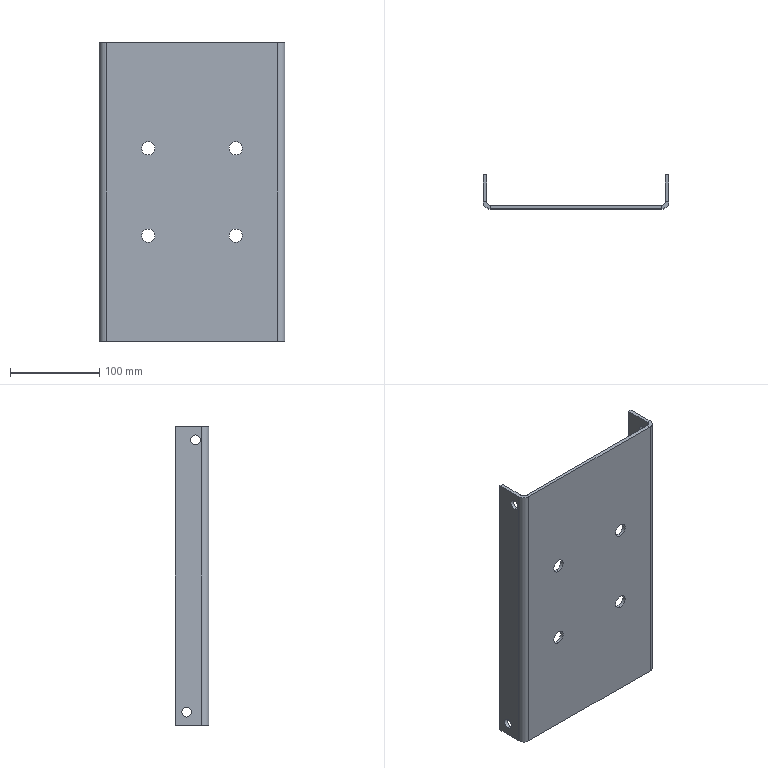Part | SolidWorks | features Cut 1, FlatPattern 1, ICE 1, SMBaseFlange 1, SheetMetal 1 | 1 solid | 38 faces | box 208 x 38 x 335 mm | volume 358590 mm3 | cylinder 20 | plane 18 | commonest cylinder face diameters 11 x8 15 x8 8 x2 16 x2
STEP:
#1=CARTESIAN_POINT('',(-49.,0.,-56.5));
#2=VERTEX_POINT('',#1);
#3=CARTESIAN_POINT('',(-49.,0.,-41.5));
#4=VERTEX_POINT('',#3);
#5=CARTESIAN_POINT('',(-49.,0.,-49.));
#6=DIRECTION('',(0.,1.,0.));
#7=DIRECTION('',(0.,0.,1.));
#8=AXIS2_PLACEMENT_3D('',#5,#6,#7);
#9=CIRCLE('',#8,7.5);
#10=EDGE_CURVE('',#2,#4,#9,.T.);
#11=ORIENTED_EDGE('',*,*,#10,.F.);
#12=CARTESIAN_POINT('',(-49.,4.,-56.5));
#13=VERTEX_POINT('',#12);
#14=CARTESIAN_POINT('',(-49.,-6.,-56.5));
#15=DIRECTION('',(0.,1.,0.));
#16=VECTOR('',#15,1000.);
#17=LINE('',#14,#16);
#18=EDGE_CURVE('',#2,#13,#17,.T.);
#19=ORIENTED_EDGE('',*,*,#18,.T.);
#20=CARTESIAN_POINT('',(-49.,4.,-41.5));
#21=VERTEX_POINT('',#20);
#22=CARTESIAN_POINT('',(-49.,4.,-49.));
#23=DIRECTION('',(0.,1.,0.));
#24=DIRECTION('',(0.,0.,1.));
#25=AXIS2_PLACEMENT_3D('',#22,#23,#24);
#26=CIRCLE('',#25,7.5);
#27=EDGE_CURVE('',#13,#21,#26,.T.);
#28=ORIENTED_EDGE('',*,*,#27,.T.);
#29=CARTESIAN_POINT('',(-49.,-6.,-41.5));
#30=DIRECTION('',(0.,1.,0.));
#31=VECTOR('',#30,1000.);
#32=LINE('',#29,#31);
#33=EDGE_CURVE('',#4,#21,#32,.T.);
#34=ORIENTED_EDGE('',*,*,#33,.F.);
#35=EDGE_LOOP('',(#11,#19,#28,#34));
#36=FACE_OUTER_BOUND('',#35,.T.);
#37=CARTESIAN_POINT('',(-49.,-6.,-49.));
#38=DIRECTION('',(0.,1.,0.));
#39=DIRECTION('',(0.,0.,1.));
#40=AXIS2_PLACEMENT_3D('',#37,#38,#39);
#41=CYLINDRICAL_SURFACE('',#40,7.5);
#42=ADVANCED_FACE('',(#36),#41,.F.);
#43=CARTESIAN_POINT('',(49.,0.,41.5));
#44=VERTEX_POINT('',#43);
#45=CARTESIAN_POINT('',(49.,0.,56.5));
#46=VERTEX_POINT('',#45);
#47=CARTESIAN_POINT('',(49.,0.,49.));
#48=DIRECTION('',(0.,1.,0.));
#49=DIRECTION('',(0.,0.,1.));
#50=AXIS2_PLACEMENT_3D('',#47,#48,#49);
#51=CIRCLE('',#50,7.5);
#52=EDGE_CURVE('',#44,#46,#51,.T.);
#53=ORIENTED_EDGE('',*,*,#52,.F.);
#54=CARTESIAN_POINT('',(49.,4.,41.5));
#55=VERTEX_POINT('',#54);
#56=CARTESIAN_POINT('',(49.,-6.,41.5));
#57=DIRECTION('',(0.,1.,0.));
#58=VECTOR('',#57,1000.);
#59=LINE('',#56,#58);
#60=EDGE_CURVE('',#44,#55,#59,.T.);
#61=ORIENTED_EDGE('',*,*,#60,.T.);
#62=CARTESIAN_POINT('',(49.,4.,56.5));
#63=VERTEX_POINT('',#62);
#64=CARTESIAN_POINT('',(49.,4.,49.));
#65=DIRECTION('',(0.,1.,0.));
#66=DIRECTION('',(0.,0.,1.));
#67=AXIS2_PLACEMENT_3D('',#64,#65,#66);
#68=CIRCLE('',#67,7.5);
#69=EDGE_CURVE('',#55,#63,#68,.T.);
#70=ORIENTED_EDGE('',*,*,#69,.T.);
#71=CARTESIAN_POINT('',(49.,-6.,56.5));
#72=DIRECTION('',(0.,1.,0.));
#73=VECTOR('',#72,1000.);
#74=LINE('',#71,#73);
#75=EDGE_CURVE('',#46,#63,#74,.T.);
#76=ORIENTED_EDGE('',*,*,#75,.F.);
#77=EDGE_LOOP('',(#53,#61,#70,#76));
#78=FACE_OUTER_BOUND('',#77,.T.);
#79=CARTESIAN_POINT('',(49.,-6.,49.));
#80=DIRECTION('',(0.,1.,0.));
#81=DIRECTION('',(0.,0.,1.));
#82=AXIS2_PLACEMENT_3D('',#79,#80,#81);
#83=CYLINDRICAL_SURFACE('',#82,7.5);
#84=ADVANCED_FACE('',(#78),#83,.F.);
#85=CARTESIAN_POINT('',(-49.,0.,41.5));
#86=VERTEX_POINT('',#85);
#87=CARTESIAN_POINT('',(-49.,0.,56.5));
#88=VERTEX_POINT('',#87);
#89=CARTESIAN_POINT('',(-49.,0.,49.));
#90=DIRECTION('',(0.,1.,0.));
#91=DIRECTION('',(0.,0.,1.));
#92=AXIS2_PLACEMENT_3D('',#89,#90,#91);
#93=CIRCLE('',#92,7.5);
#94=EDGE_CURVE('',#86,#88,#93,.T.);
#95=ORIENTED_EDGE('',*,*,#94,.F.);
#96=CARTESIAN_POINT('',(-49.,4.,41.5));
#97=VERTEX_POINT('',#96);
#98=CARTESIAN_POINT('',(-49.,-6.,41.5));
#99=DIRECTION('',(0.,1.,0.));
#100=VECTOR('',#99,1000.);
#101=LINE('',#98,#100);
#102=EDGE_CURVE('',#86,#97,#101,.T.);
#103=ORIENTED_EDGE('',*,*,#102,.T.);
#104=CARTESIAN_POINT('',(-49.,4.,56.5));
#105=VERTEX_POINT('',#104);
#106=CARTESIAN_POINT('',(-49.,4.,49.));
#107=DIRECTION('',(0.,1.,0.));
#108=DIRECTION('',(0.,0.,1.));
#109=AXIS2_PLACEMENT_3D('',#106,#107,#108);
#110=CIRCLE('',#109,7.5);
#111=EDGE_CURVE('',#97,#105,#110,.T.);
#112=ORIENTED_EDGE('',*,*,#111,.T.);
#113=CARTESIAN_POINT('',(-49.,-6.,56.5));
#114=DIRECTION('',(0.,1.,0.));
#115=VECTOR('',#114,1000.);
#116=LINE('',#113,#115);
#117=EDGE_CURVE('',#88,#105,#116,.T.);
#118=ORIENTED_EDGE('',*,*,#117,.F.);
#119=EDGE_LOOP('',(#95,#103,#112,#118));
#120=FACE_OUTER_BOUND('',#119,.T.);
#121=CARTESIAN_POINT('',(-49.,-6.,49.));
#122=DIRECTION('',(0.,1.,0.));
#123=DIRECTION('',(0.,0.,1.));
#124=AXIS2_PLACEMENT_3D('',#121,#122,#123);
#125=CYLINDRICAL_SURFACE('',#124,7.5);
#126=ADVANCED_FACE('',(#120),#125,.F.);
#127=CARTESIAN_POINT('',(49.,0.,-56.5));
#128=VERTEX_POINT('',#127);
#129=CARTESIAN_POINT('',(49.,0.,-41.5));
#130=VERTEX_POINT('',#129);
#131=CARTESIAN_POINT('',(49.,0.,-49.));
#132=DIRECTION('',(0.,1.,0.));
#133=DIRECTION('',(0.,0.,1.));
#134=AXIS2_PLACEMENT_3D('',#131,#132,#133);
#135=CIRCLE('',#134,7.5);
#136=EDGE_CURVE('',#128,#130,#135,.T.);
#137=ORIENTED_EDGE('',*,*,#136,.F.);
#138=CARTESIAN_POINT('',(49.,4.,-56.5));
#139=VERTEX_POINT('',#138);
#140=CARTESIAN_POINT('',(49.,-6.,-56.5));
#141=DIRECTION('',(0.,1.,0.));
#142=VECTOR('',#141,1000.);
#143=LINE('',#140,#142);
#144=EDGE_CURVE('',#128,#139,#143,.T.);
#145=ORIENTED_EDGE('',*,*,#144,.T.);
#146=CARTESIAN_POINT('',(49.,4.,-41.5));
#147=VERTEX_POINT('',#146);
#148=CARTESIAN_POINT('',(49.,4.,-49.));
#149=DIRECTION('',(0.,1.,0.));
#150=DIRECTION('',(0.,0.,1.));
#151=AXIS2_PLACEMENT_3D('',#148,#149,#150);
#152=CIRCLE('',#151,7.5);
#153=EDGE_CURVE('',#139,#147,#152,.T.);
#154=ORIENTED_EDGE('',*,*,#153,.T.);
#155=CARTESIAN_POINT('',(49.,-6.,-41.5));
#156=DIRECTION('',(0.,1.,0.));
#157=VECTOR('',#156,1000.);
#158=LINE('',#155,#157);
#159=EDGE_CURVE('',#130,#147,#158,.T.);
#160=ORIENTED_EDGE('',*,*,#159,.F.);
#161=EDGE_LOOP('',(#137,#145,#154,#160));
#162=FACE_OUTER_BOUND('',#161,.T.);
#163=CARTESIAN_POINT('',(49.,-6.,-49.));
#164=DIRECTION('',(0.,1.,0.));
#165=DIRECTION('',(0.,0.,1.));
#166=AXIS2_PLACEMENT_3D('',#163,#164,#165);
#167=CYLINDRICAL_SURFACE('',#166,7.5);
#168=ADVANCED_FACE('',(#162),#167,.F.);
#169=CARTESIAN_POINT('',(104.,25.,-158.));
#170=VERTEX_POINT('',#169);
#171=CARTESIAN_POINT('',(104.,25.,-147.));
#172=VERTEX_POINT('',#171);
#173=CARTESIAN_POINT('',(104.,25.,-152.5));
#174=DIRECTION('',(-1.,0.,0.));
#175=DIRECTION('',(0.,0.,1.));
#176=AXIS2_PLACEMENT_3D('',#173,#174,#175);
#177=CIRCLE('',#176,5.5);
#178=EDGE_CURVE('',#170,#172,#177,.T.);
#179=ORIENTED_EDGE('',*,*,#178,.F.);
#180=CARTESIAN_POINT('',(100.,25.,-158.));
#181=VERTEX_POINT('',#180);
#182=CARTESIAN_POINT('',(104.,25.,-158.));
#183=DIRECTION('',(-1.,0.,0.));
#184=VECTOR('',#183,1000.);
#185=LINE('',#182,#184);
#186=EDGE_CURVE('',#170,#181,#185,.T.);
#187=ORIENTED_EDGE('',*,*,#186,.T.);
#188=CARTESIAN_POINT('',(100.,25.,-147.));
#189=VERTEX_POINT('',#188);
#190=CARTESIAN_POINT('',(100.,25.,-152.5));
#191=DIRECTION('',(-1.,0.,0.));
#192=DIRECTION('',(0.,0.,1.));
#193=AXIS2_PLACEMENT_3D('',#190,#191,#192);
#194=CIRCLE('',#193,5.5);
#195=EDGE_CURVE('',#181,#189,#194,.T.);
#196=ORIENTED_EDGE('',*,*,#195,.T.);
#197=CARTESIAN_POINT('',(104.,25.,-147.));
#198=DIRECTION('',(-1.,0.,0.));
#199=VECTOR('',#198,1000.);
#200=LINE('',#197,#199);
#201=EDGE_CURVE('',#172,#189,#200,.T.);
#202=ORIENTED_EDGE('',*,*,#201,.F.);
#203=EDGE_LOOP('',(#179,#187,#196,#202));
#204=FACE_OUTER_BOUND('',#203,.T.);
#205=CARTESIAN_POINT('',(104.,25.,-152.5));
#206=DIRECTION('',(-1.,0.,0.));
#207=DIRECTION('',(0.,0.,1.));
#208=AXIS2_PLACEMENT_3D('',#205,#206,#207);
#209=CYLINDRICAL_SURFACE('',#208,5.5);
#210=ADVANCED_FACE('',(#204),#209,.F.);
#211=CARTESIAN_POINT('',(104.,15.,147.));
#212=VERTEX_POINT('',#211);
#213=CARTESIAN_POINT('',(104.,15.,158.));
#214=VERTEX_POINT('',#213);
#215=CARTESIAN_POINT('',(104.,15.,152.5));
#216=DIRECTION('',(-1.,0.,0.));
#217=DIRECTION('',(0.,0.,1.));
#218=AXIS2_PLACEMENT_3D('',#215,#216,#217);
#219=CIRCLE('',#218,5.5);
#220=EDGE_CURVE('',#212,#214,#219,.T.);
#221=ORIENTED_EDGE('',*,*,#220,.F.);
#222=CARTESIAN_POINT('',(100.,15.,147.));
#223=VERTEX_POINT('',#222);
#224=CARTESIAN_POINT('',(104.,15.,147.));
#225=DIRECTION('',(-1.,0.,0.));
#226=VECTOR('',#225,1000.);
#227=LINE('',#224,#226);
#228=EDGE_CURVE('',#212,#223,#227,.T.);
#229=ORIENTED_EDGE('',*,*,#228,.T.);
#230=CARTESIAN_POINT('',(100.,15.,158.));
#231=VERTEX_POINT('',#230);
#232=CARTESIAN_POINT('',(100.,15.,152.5));
#233=DIRECTION('',(-1.,0.,0.));
#234=DIRECTION('',(0.,0.,1.));
#235=AXIS2_PLACEMENT_3D('',#232,#233,#234);
#236=CIRCLE('',#235,5.5);
#237=EDGE_CURVE('',#223,#231,#236,.T.);
#238=ORIENTED_EDGE('',*,*,#237,.T.);
#239=CARTESIAN_POINT('',(104.,15.,158.));
#240=DIRECTION('',(-1.,0.,0.));
#241=VECTOR('',#240,1000.);
#242=LINE('',#239,#241);
#243=EDGE_CURVE('',#214,#231,#242,.T.);
#244=ORIENTED_EDGE('',*,*,#243,.F.);
#245=EDGE_LOOP('',(#221,#229,#238,#244));
#246=FACE_OUTER_BOUND('',#245,.T.);
#247=CARTESIAN_POINT('',(104.,15.,152.5));
#248=DIRECTION('',(-1.,0.,0.));
#249=DIRECTION('',(0.,0.,1.));
#250=AXIS2_PLACEMENT_3D('',#247,#248,#249);
#251=CYLINDRICAL_SURFACE('',#250,5.5);
#252=ADVANCED_FACE('',(#246),#251,.F.);
#253=CARTESIAN_POINT('',(-100.,25.,-147.));
#254=VERTEX_POINT('',#253);
#255=CARTESIAN_POINT('',(-100.,25.,-158.));
#256=VERTEX_POINT('',#255);
#257=CARTESIAN_POINT('',(-100.,25.,-152.5));
#258=DIRECTION('',(1.,0.,0.));
#259=DIRECTION('',(0.,0.,-1.));
#260=AXIS2_PLACEMENT_3D('',#257,#258,#259);
#261=CIRCLE('',#260,5.5);
#262=EDGE_CURVE('',#254,#256,#261,.T.);
#263=ORIENTED_EDGE('',*,*,#262,.T.);
#264=CARTESIAN_POINT('',(-104.,25.,-158.));
#265=VERTEX_POINT('',#264);
#266=CARTESIAN_POINT('',(104.,25.,-158.));
#267=DIRECTION('',(-1.,0.,0.));
#268=VECTOR('',#267,1000.);
#269=LINE('',#266,#268);
#270=EDGE_CURVE('',#256,#265,#269,.T.);
#271=ORIENTED_EDGE('',*,*,#270,.T.);
#272=CARTESIAN_POINT('',(-104.,25.,-147.));
#273=VERTEX_POINT('',#272);
#274=CARTESIAN_POINT('',(-104.,25.,-152.5));
#275=DIRECTION('',(1.,0.,0.));
#276=DIRECTION('',(0.,0.,-1.));
#277=AXIS2_PLACEMENT_3D('',#274,#275,#276);
#278=CIRCLE('',#277,5.5);
#279=EDGE_CURVE('',#273,#265,#278,.T.);
#280=ORIENTED_EDGE('',*,*,#279,.F.);
#281=CARTESIAN_POINT('',(104.,25.,-147.));
#282=DIRECTION('',(-1.,0.,0.));
#283=VECTOR('',#282,1000.);
#284=LINE('',#281,#283);
#285=EDGE_CURVE('',#254,#273,#284,.T.);
#286=ORIENTED_EDGE('',*,*,#285,.F.);
#287=EDGE_LOOP('',(#263,#271,#280,#286));
#288=FACE_OUTER_BOUND('',#287,.T.);
#289=CARTESIAN_POINT('',(104.,25.,-152.5));
#290=DIRECTION('',(-1.,0.,0.));
#291=DIRECTION('',(0.,0.,1.));
#292=AXIS2_PLACEMENT_3D('',#289,#290,#291);
#293=CYLINDRICAL_SURFACE('',#292,5.5);
#294=ADVANCED_FACE('',(#288),#293,.F.);
#295=CARTESIAN_POINT('',(-100.,15.,158.));
#296=VERTEX_POINT('',#295);
#297=CARTESIAN_POINT('',(-100.,15.,147.));
#298=VERTEX_POINT('',#297);
#299=CARTESIAN_POINT('',(-100.,15.,152.5));
#300=DIRECTION('',(1.,0.,0.));
#301=DIRECTION('',(0.,0.,-1.));
#302=AXIS2_PLACEMENT_3D('',#299,#300,#301);
#303=CIRCLE('',#302,5.5);
#304=EDGE_CURVE('',#296,#298,#303,.T.);
#305=ORIENTED_EDGE('',*,*,#304,.T.);
#306=CARTESIAN_POINT('',(-104.,15.,147.));
#307=VERTEX_POINT('',#306);
#308=CARTESIAN_POINT('',(104.,15.,147.));
#309=DIRECTION('',(-1.,0.,0.));
#310=VECTOR('',#309,1000.);
#311=LINE('',#308,#310);
#312=EDGE_CURVE('',#298,#307,#311,.T.);
#313=ORIENTED_EDGE('',*,*,#312,.T.);
#314=CARTESIAN_POINT('',(-104.,15.,158.));
#315=VERTEX_POINT('',#314);
#316=CARTESIAN_POINT('',(-104.,15.,152.5));
#317=DIRECTION('',(1.,0.,0.));
#318=DIRECTION('',(0.,0.,-1.));
#319=AXIS2_PLACEMENT_3D('',#316,#317,#318);
#320=CIRCLE('',#319,5.5);
#321=EDGE_CURVE('',#315,#307,#320,.T.);
#322=ORIENTED_EDGE('',*,*,#321,.F.);
#323=CARTESIAN_POINT('',(104.,15.,158.));
#324=DIRECTION('',(-1.,0.,0.));
#325=VECTOR('',#324,1000.);
#326=LINE('',#323,#325);
#327=EDGE_CURVE('',#296,#315,#326,.T.);
#328=ORIENTED_EDGE('',*,*,#327,.F.);
#329=EDGE_LOOP('',(#305,#313,#322,#328));
#330=FACE_OUTER_BOUND('',#329,.T.);
#331=CARTESIAN_POINT('',(104.,15.,152.5));
#332=DIRECTION('',(-1.,0.,0.));
#333=DIRECTION('',(0.,0.,1.));
#334=AXIS2_PLACEMENT_3D('',#331,#332,#333);
#335=CYLINDRICAL_SURFACE('',#334,5.5);
#336=ADVANCED_FACE('',(#330),#335,.F.);
#337=CARTESIAN_POINT('',(-104.,8.,167.5));
#338=VERTEX_POINT('',#337);
#339=CARTESIAN_POINT('',(-100.,8.,167.5));
#340=VERTEX_POINT('',#339);
#341=CARTESIAN_POINT('',(-104.,8.,167.5));
#342=DIRECTION('',(1.,0.,0.));
#343=VECTOR('',#342,1000.);
#344=LINE('',#341,#343);
#345=EDGE_CURVE('',#338,#340,#344,.T.);
#346=ORIENTED_EDGE('',*,*,#345,.F.);
#347=CARTESIAN_POINT('',(-96.,0.,167.5));
#348=VERTEX_POINT('',#347);
#349=CARTESIAN_POINT('',(-96.,8.,167.5));
#350=DIRECTION('',(0.,0.,1.));
#351=DIRECTION('',(-1.,0.,0.));
#352=AXIS2_PLACEMENT_3D('',#349,#350,#351);
#353=CIRCLE('',#352,8.);
#354=EDGE_CURVE('',#338,#348,#353,.T.);
#355=ORIENTED_EDGE('',*,*,#354,.T.);
#356=CARTESIAN_POINT('',(-96.,4.,167.5));
#357=VERTEX_POINT('',#356);
#358=CARTESIAN_POINT('',(-96.,4.,167.5));
#359=DIRECTION('',(0.,-1.,0.));
#360=VECTOR('',#359,1000.);
#361=LINE('',#358,#360);
#362=EDGE_CURVE('',#357,#348,#361,.T.);
#363=ORIENTED_EDGE('',*,*,#362,.F.);
#364=CARTESIAN_POINT('',(-96.,8.,167.5));
#365=DIRECTION('',(0.,0.,1.));
#366=DIRECTION('',(1.,0.,0.));
#367=AXIS2_PLACEMENT_3D('',#364,#365,#366);
#368=CIRCLE('',#367,4.);
#369=EDGE_CURVE('',#340,#357,#368,.T.);
#370=ORIENTED_EDGE('',*,*,#369,.F.);
#371=EDGE_LOOP('',(#346,#355,#363,#370));
#372=FACE_OUTER_BOUND('',#371,.T.);
#373=CARTESIAN_POINT('',(-104.,8.,167.5));
#374=DIRECTION('',(0.,0.,1.));
#375=DIRECTION('',(1.,0.,0.));
#376=AXIS2_PLACEMENT_3D('',#373,#374,#375);
#377=PLANE('',#376);
#378=ADVANCED_FACE('',(#372),#377,.T.);
#379=CARTESIAN_POINT('',(-104.,38.,167.5));
#380=VERTEX_POINT('',#379);
#381=CARTESIAN_POINT('',(-104.,38.,167.5));
#382=DIRECTION('',(0.,-1.,0.));
#383=VECTOR('',#382,1000.);
#384=LINE('',#381,#383);
#385=EDGE_CURVE('',#380,#338,#384,.T.);
#386=ORIENTED_EDGE('',*,*,#385,.T.);
#387=ORIENTED_EDGE('',*,*,#345,.T.);
#388=CARTESIAN_POINT('',(-100.,38.,167.5));
#389=VERTEX_POINT('',#388);
#390=CARTESIAN_POINT('',(-100.,38.,167.5));
#391=DIRECTION('',(0.,-1.,0.));
#392=VECTOR('',#391,1000.);
#393=LINE('',#390,#392);
#394=EDGE_CURVE('',#389,#340,#393,.T.);
#395=ORIENTED_EDGE('',*,*,#394,.F.);
#396=CARTESIAN_POINT('',(-104.,38.,167.5));
#397=DIRECTION('',(1.,0.,0.));
#398=VECTOR('',#397,1000.);
#399=LINE('',#396,#398);
#400=EDGE_CURVE('',#380,#389,#399,.T.);
#401=ORIENTED_EDGE('',*,*,#400,.F.);
#402=EDGE_LOOP('',(#386,#387,#395,#401));
#403=FACE_OUTER_BOUND('',#402,.T.);
#404=CARTESIAN_POINT('',(-96.,4.,167.5));
#405=DIRECTION('',(0.,0.,1.));
#406=DIRECTION('',(1.,0.,0.));
#407=AXIS2_PLACEMENT_3D('',#404,#405,#406);
#408=PLANE('',#407);
#409=ADVANCED_FACE('',(#403),#408,.T.);
#410=CARTESIAN_POINT('',(-96.,0.,-167.5));
#411=VERTEX_POINT('',#410);
#412=CARTESIAN_POINT('',(-96.,4.,-167.5));
#413=VERTEX_POINT('',#412);
#414=CARTESIAN_POINT('',(-96.,0.,-167.5));
#415=DIRECTION('',(0.,1.,0.));
#416=VECTOR('',#415,1000.);
#417=LINE('',#414,#416);
#418=EDGE_CURVE('',#411,#413,#417,.T.);
#419=ORIENTED_EDGE('',*,*,#418,.F.);
#420=CARTESIAN_POINT('',(-104.,8.,-167.5));
#421=VERTEX_POINT('',#420);
#422=CARTESIAN_POINT('',(-96.,8.,-167.5));
#423=DIRECTION('',(0.,0.,1.));
#424=DIRECTION('',(-1.,0.,0.));
#425=AXIS2_PLACEMENT_3D('',#422,#423,#424);
#426=CIRCLE('',#425,8.);
#427=EDGE_CURVE('',#421,#411,#426,.T.);
#428=ORIENTED_EDGE('',*,*,#427,.F.);
#429=CARTESIAN_POINT('',(-100.,8.,-167.5));
#430=VERTEX_POINT('',#429);
#431=CARTESIAN_POINT('',(-100.,8.,-167.5));
#432=DIRECTION('',(-1.,0.,0.));
#433=VECTOR('',#432,1000.);
#434=LINE('',#431,#433);
#435=EDGE_CURVE('',#430,#421,#434,.T.);
#436=ORIENTED_EDGE('',*,*,#435,.F.);
#437=CARTESIAN_POINT('',(-96.,8.,-167.5));
#438=DIRECTION('',(0.,0.,1.));
#439=DIRECTION('',(1.,0.,0.));
#440=AXIS2_PLACEMENT_3D('',#437,#438,#439);
#441=CIRCLE('',#440,4.);
#442=EDGE_CURVE('',#430,#413,#441,.T.);
#443=ORIENTED_EDGE('',*,*,#442,.T.);
#444=EDGE_LOOP('',(#419,#428,#436,#443));
#445=FACE_OUTER_BOUND('',#444,.T.);
#446=CARTESIAN_POINT('',(-96.,0.,-167.5));
#447=DIRECTION('',(0.,0.,-1.));
#448=DIRECTION('',(-1.,0.,0.));
#449=AXIS2_PLACEMENT_3D('',#446,#447,#448);
#450=PLANE('',#449);
#451=ADVANCED_FACE('',(#445),#450,.T.);
#452=CARTESIAN_POINT('',(96.,0.,-167.5));
#453=VERTEX_POINT('',#452);
#454=CARTESIAN_POINT('',(-104.,0.,-167.5));
#455=DIRECTION('',(1.,0.,0.));
#456=VECTOR('',#455,1000.);
#457=LINE('',#454,#456);
#458=EDGE_CURVE('',#411,#453,#457,.T.);
#459=ORIENTED_EDGE('',*,*,#458,.F.);
#460=ORIENTED_EDGE('',*,*,#418,.T.);
#461=CARTESIAN_POINT('',(96.,4.,-167.5));
#462=VERTEX_POINT('',#461);
#463=CARTESIAN_POINT('',(-104.,4.,-167.5));
#464=DIRECTION('',(1.,0.,0.));
#465=VECTOR('',#464,1000.);
#466=LINE('',#463,#465);
#467=EDGE_CURVE('',#413,#462,#466,.T.);
#468=ORIENTED_EDGE('',*,*,#467,.T.);
#469=CARTESIAN_POINT('',(96.,4.,-167.5));
#470=DIRECTION('',(0.,-1.,0.));
#471=VECTOR('',#470,1000.);
#472=LINE('',#469,#471);
#473=EDGE_CURVE('',#462,#453,#472,.T.);
#474=ORIENTED_EDGE('',*,*,#473,.T.);
#475=EDGE_LOOP('',(#459,#460,#468,#474));
#476=FACE_OUTER_BOUND('',#475,.T.);
#477=CARTESIAN_POINT('',(-100.,8.,-167.5));
#478=DIRECTION('',(0.,0.,-1.));
#479=DIRECTION('',(-1.,0.,0.));
#480=AXIS2_PLACEMENT_3D('',#477,#478,#479);
#481=PLANE('',#480);
#482=ADVANCED_FACE('',(#476),#481,.T.);
#483=CARTESIAN_POINT('',(96.,0.,167.5));
#484=VERTEX_POINT('',#483);
#485=CARTESIAN_POINT('',(96.,4.,167.5));
#486=VERTEX_POINT('',#485);
#487=CARTESIAN_POINT('',(96.,0.,167.5));
#488=DIRECTION('',(0.,1.,0.));
#489=VECTOR('',#488,1000.);
#490=LINE('',#487,#489);
#491=EDGE_CURVE('',#484,#486,#490,.T.);
#492=ORIENTED_EDGE('',*,*,#491,.F.);
#493=CARTESIAN_POINT('',(104.,8.,167.5));
#494=VERTEX_POINT('',#493);
#495=CARTESIAN_POINT('',(96.,8.,167.5));
#496=DIRECTION('',(0.,0.,1.));
#497=DIRECTION('',(-1.,0.,0.));
#498=AXIS2_PLACEMENT_3D('',#495,#496,#497);
#499=CIRCLE('',#498,8.);
#500=EDGE_CURVE('',#484,#494,#499,.T.);
#501=ORIENTED_EDGE('',*,*,#500,.T.);
#502=CARTESIAN_POINT('',(100.,8.,167.5));
#503=VERTEX_POINT('',#502);
#504=CARTESIAN_POINT('',(100.,8.,167.5));
#505=DIRECTION('',(1.,0.,0.));
#506=VECTOR('',#505,1000.);
#507=LINE('',#504,#506);
#508=EDGE_CURVE('',#503,#494,#507,.T.);
#509=ORIENTED_EDGE('',*,*,#508,.F.);
#510=CARTESIAN_POINT('',(96.,8.,167.5));
#511=DIRECTION('',(0.,0.,1.));
#512=DIRECTION('',(1.,0.,0.));
#513=AXIS2_PLACEMENT_3D('',#510,#511,#512);
#514=CIRCLE('',#513,4.);
#515=EDGE_CURVE('',#486,#503,#514,.T.);
#516=ORIENTED_EDGE('',*,*,#515,.F.);
#517=EDGE_LOOP('',(#492,#501,#509,#516));
#518=FACE_OUTER_BOUND('',#517,.T.);
#519=CARTESIAN_POINT('',(96.,0.,167.5));
#520=DIRECTION('',(0.,0.,1.));
#521=DIRECTION('',(1.,0.,0.));
#522=AXIS2_PLACEMENT_3D('',#519,#520,#521);
#523=PLANE('',#522);
#524=ADVANCED_FACE('',(#518),#523,.T.);
#525=CARTESIAN_POINT('',(-104.,0.,167.5));
#526=DIRECTION('',(1.,0.,0.));
#527=VECTOR('',#526,1000.);
#528=LINE('',#525,#527);
#529=EDGE_CURVE('',#348,#484,#528,.T.);
#530=ORIENTED_EDGE('',*,*,#529,.T.);
#531=ORIENTED_EDGE('',*,*,#491,.T.);
#532=CARTESIAN_POINT('',(-104.,4.,167.5));
#533=DIRECTION('',(1.,0.,0.));
#534=VECTOR('',#533,1000.);
#535=LINE('',#532,#534);
#536=EDGE_CURVE('',#357,#486,#535,.T.);
#537=ORIENTED_EDGE('',*,*,#536,.F.);
#538=ORIENTED_EDGE('',*,*,#362,.T.);
#539=EDGE_LOOP('',(#530,#531,#537,#538));
#540=FACE_OUTER_BOUND('',#539,.T.);
#541=CARTESIAN_POINT('',(100.,8.,167.5));
#542=DIRECTION('',(0.,0.,1.));
#543=DIRECTION('',(1.,0.,0.));
#544=AXIS2_PLACEMENT_3D('',#541,#542,#543);
#545=PLANE('',#544);
#546=ADVANCED_FACE('',(#540),#545,.T.);
#547=CARTESIAN_POINT('',(104.,8.,-167.5));
#548=VERTEX_POINT('',#547);
#549=CARTESIAN_POINT('',(100.,8.,-167.5));
#550=VERTEX_POINT('',#549);
#551=CARTESIAN_POINT('',(104.,8.,-167.5));
#552=DIRECTION('',(-1.,0.,0.));
#553=VECTOR('',#552,1000.);
#554=LINE('',#551,#553);
#555=EDGE_CURVE('',#548,#550,#554,.T.);
#556=ORIENTED_EDGE('',*,*,#555,.F.);
#557=CARTESIAN_POINT('',(96.,8.,-167.5));
#558=DIRECTION('',(0.,0.,1.));
#559=DIRECTION('',(-1.,0.,0.));
#560=AXIS2_PLACEMENT_3D('',#557,#558,#559);
#561=CIRCLE('',#560,8.);
#562=EDGE_CURVE('',#453,#548,#561,.T.);
#563=ORIENTED_EDGE('',*,*,#562,.F.);
#564=ORIENTED_EDGE('',*,*,#473,.F.);
#565=CARTESIAN_POINT('',(96.,8.,-167.5));
#566=DIRECTION('',(0.,0.,1.));
#567=DIRECTION('',(1.,0.,0.));
#568=AXIS2_PLACEMENT_3D('',#565,#566,#567);
#569=CIRCLE('',#568,4.);
#570=EDGE_CURVE('',#462,#550,#569,.T.);
#571=ORIENTED_EDGE('',*,*,#570,.T.);
#572=EDGE_LOOP('',(#556,#563,#564,#571));
#573=FACE_OUTER_BOUND('',#572,.T.);
#574=CARTESIAN_POINT('',(104.,8.,-167.5));
#575=DIRECTION('',(0.,0.,-1.));
#576=DIRECTION('',(-1.,0.,0.));
#577=AXIS2_PLACEMENT_3D('',#574,#575,#576);
#578=PLANE('',#577);
#579=ADVANCED_FACE('',(#573),#578,.T.);
#580=CARTESIAN_POINT('',(104.,38.,-167.5));
#581=VERTEX_POINT('',#580);
#582=CARTESIAN_POINT('',(104.,0.,-167.5));
#583=DIRECTION('',(0.,1.,0.));
#584=VECTOR('',#583,1000.);
#585=LINE('',#582,#584);
#586=EDGE_CURVE('',#548,#581,#585,.T.);
#587=ORIENTED_EDGE('',*,*,#586,.F.);
#588=ORIENTED_EDGE('',*,*,#555,.T.);
#589=CARTESIAN_POINT('',(100.,38.,-167.5));
#590=VERTEX_POINT('',#589);
#591=CARTESIAN_POINT('',(100.,0.,-167.5));
#592=DIRECTION('',(0.,1.,0.));
#593=VECTOR('',#592,1000.);
#594=LINE('',#591,#593);
#595=EDGE_CURVE('',#550,#590,#594,.T.);
#596=ORIENTED_EDGE('',*,*,#595,.T.);
#597=CARTESIAN_POINT('',(100.,38.,-167.5));
#598=DIRECTION('',(1.,0.,0.));
#599=VECTOR('',#598,1000.);
#600=LINE('',#597,#599);
#601=EDGE_CURVE('',#590,#581,#600,.T.);
#602=ORIENTED_EDGE('',*,*,#601,.T.);
#603=EDGE_LOOP('',(#587,#588,#596,#602));
#604=FACE_OUTER_BOUND('',#603,.T.);
#605=CARTESIAN_POINT('',(96.,4.,-167.5));
#606=DIRECTION('',(0.,0.,-1.));
#607=DIRECTION('',(-1.,0.,0.));
#608=AXIS2_PLACEMENT_3D('',#605,#606,#607);
#609=PLANE('',#608);
#610=ADVANCED_FACE('',(#604),#609,.T.);
#611=CARTESIAN_POINT('',(104.,25.,-152.5));
#612=DIRECTION('',(-1.,0.,0.));
#613=DIRECTION('',(0.,0.,1.));
#614=AXIS2_PLACEMENT_3D('',#611,#612,#613);
#615=CIRCLE('',#614,5.5);
#616=EDGE_CURVE('',#172,#170,#615,.T.);
#617=ORIENTED_EDGE('',*,*,#616,.T.);
#618=ORIENTED_EDGE('',*,*,#178,.T.);
#619=EDGE_LOOP('',(#617,#618));
#620=FACE_BOUND('',#619,.T.);
#621=CARTESIAN_POINT('',(104.,15.,152.5));
#622=DIRECTION('',(-1.,0.,0.));
#623=DIRECTION('',(0.,0.,1.));
#624=AXIS2_PLACEMENT_3D('',#621,#622,#623);
#625=CIRCLE('',#624,5.5);
#626=EDGE_CURVE('',#214,#212,#625,.T.);
#627=ORIENTED_EDGE('',*,*,#626,.T.);
#628=ORIENTED_EDGE('',*,*,#220,.T.);
#629=EDGE_LOOP('',(#627,#628));
#630=FACE_BOUND('',#629,.T.);
#631=ORIENTED_EDGE('',*,*,#586,.T.);
#632=CARTESIAN_POINT('',(104.,38.,167.5));
#633=VERTEX_POINT('',#632);
#634=CARTESIAN_POINT('',(104.,38.,167.5));
#635=DIRECTION('',(0.,0.,-1.));
#636=VECTOR('',#635,1000.);
#637=LINE('',#634,#636);
#638=EDGE_CURVE('',#633,#581,#637,.T.);
#639=ORIENTED_EDGE('',*,*,#638,.F.);
#640=CARTESIAN_POINT('',(104.,0.,167.5));
#641=DIRECTION('',(0.,1.,0.));
#642=VECTOR('',#641,1000.);
#643=LINE('',#640,#642);
#644=EDGE_CURVE('',#494,#633,#643,.T.);
#645=ORIENTED_EDGE('',*,*,#644,.F.);
#646=CARTESIAN_POINT('',(104.,8.,167.5));
#647=DIRECTION('',(0.,0.,-1.));
#648=VECTOR('',#647,1000.);
#649=LINE('',#646,#648);
#650=EDGE_CURVE('',#494,#548,#649,.T.);
#651=ORIENTED_EDGE('',*,*,#650,.T.);
#652=EDGE_LOOP('',(#631,#639,#645,#651));
#653=FACE_OUTER_BOUND('',#652,.T.);
#654=CARTESIAN_POINT('',(104.,0.,167.5));
#655=DIRECTION('',(-1.,0.,0.));
#656=DIRECTION('',(0.,0.,1.));
#657=AXIS2_PLACEMENT_3D('',#654,#655,#656);
#658=PLANE('',#657);
#659=ADVANCED_FACE('',(#620,#630,#653),#658,.F.);
#660=ORIENTED_EDGE('',*,*,#601,.F.);
#661=CARTESIAN_POINT('',(100.,38.,167.5));
#662=VERTEX_POINT('',#661);
#663=CARTESIAN_POINT('',(100.,38.,167.5));
#664=DIRECTION('',(0.,0.,-1.));
#665=VECTOR('',#664,1000.);
#666=LINE('',#663,#665);
#667=EDGE_CURVE('',#662,#590,#666,.T.);
#668=ORIENTED_EDGE('',*,*,#667,.F.);
#669=CARTESIAN_POINT('',(100.,38.,167.5));
#670=DIRECTION('',(1.,0.,0.));
#671=VECTOR('',#670,1000.);
#672=LINE('',#669,#671);
#673=EDGE_CURVE('',#662,#633,#672,.T.);
#674=ORIENTED_EDGE('',*,*,#673,.T.);
#675=ORIENTED_EDGE('',*,*,#638,.T.);
#676=EDGE_LOOP('',(#660,#668,#674,#675));
#677=FACE_OUTER_BOUND('',#676,.T.);
#678=CARTESIAN_POINT('',(100.,38.,167.5));
#679=DIRECTION('',(0.,1.,0.));
#680=DIRECTION('',(0.,0.,1.));
#681=AXIS2_PLACEMENT_3D('',#678,#679,#680);
#682=PLANE('',#681);
#683=ADVANCED_FACE('',(#677),#682,.T.);
#684=CARTESIAN_POINT('',(100.,25.,-152.5));
#685=DIRECTION('',(-1.,0.,0.));
#686=DIRECTION('',(0.,0.,1.));
#687=AXIS2_PLACEMENT_3D('',#684,#685,#686);
#688=CIRCLE('',#687,5.5);
#689=EDGE_CURVE('',#189,#181,#688,.T.);
#690=ORIENTED_EDGE('',*,*,#689,.F.);
#691=ORIENTED_EDGE('',*,*,#195,.F.);
#692=EDGE_LOOP('',(#690,#691));
#693=FACE_BOUND('',#692,.T.);
#694=CARTESIAN_POINT('',(100.,15.,152.5));
#695=DIRECTION('',(-1.,0.,0.));
#696=DIRECTION('',(0.,0.,1.));
#697=AXIS2_PLACEMENT_3D('',#694,#695,#696);
#698=CIRCLE('',#697,5.5);
#699=EDGE_CURVE('',#231,#223,#698,.T.);
#700=ORIENTED_EDGE('',*,*,#699,.F.);
#701=ORIENTED_EDGE('',*,*,#237,.F.);
#702=EDGE_LOOP('',(#700,#701));
#703=FACE_BOUND('',#702,.T.);
#704=ORIENTED_EDGE('',*,*,#595,.F.);
#705=CARTESIAN_POINT('',(100.,8.,167.5));
#706=DIRECTION('',(0.,0.,-1.));
#707=VECTOR('',#706,1000.);
#708=LINE('',#705,#707);
#709=EDGE_CURVE('',#503,#550,#708,.T.);
#710=ORIENTED_EDGE('',*,*,#709,.F.);
#711=CARTESIAN_POINT('',(100.,0.,167.5));
#712=DIRECTION('',(0.,1.,0.));
#713=VECTOR('',#712,1000.);
#714=LINE('',#711,#713);
#715=EDGE_CURVE('',#503,#662,#714,.T.);
#716=ORIENTED_EDGE('',*,*,#715,.T.);
#717=ORIENTED_EDGE('',*,*,#667,.T.);
#718=EDGE_LOOP('',(#704,#710,#716,#717));
#719=FACE_OUTER_BOUND('',#718,.T.);
#720=CARTESIAN_POINT('',(100.,0.,167.5));
#721=DIRECTION('',(-1.,0.,0.));
#722=DIRECTION('',(0.,0.,1.));
#723=AXIS2_PLACEMENT_3D('',#720,#721,#722);
#724=PLANE('',#723);
#725=ADVANCED_FACE('',(#693,#703,#719),#724,.T.);
#726=ORIENTED_EDGE('',*,*,#570,.F.);
#727=CARTESIAN_POINT('',(96.,4.,167.5));
#728=DIRECTION('',(0.,0.,-1.));
#729=VECTOR('',#728,1000.);
#730=LINE('',#727,#729);
#731=EDGE_CURVE('',#486,#462,#730,.T.);
#732=ORIENTED_EDGE('',*,*,#731,.F.);
#733=ORIENTED_EDGE('',*,*,#515,.T.);
#734=ORIENTED_EDGE('',*,*,#709,.T.);
#735=EDGE_LOOP('',(#726,#732,#733,#734));
#736=FACE_OUTER_BOUND('',#735,.T.);
#737=CARTESIAN_POINT('',(96.,8.,167.5));
#738=DIRECTION('',(0.,0.,-1.));
#739=DIRECTION('',(-1.,0.,0.));
#740=AXIS2_PLACEMENT_3D('',#737,#738,#739);
#741=CYLINDRICAL_SURFACE('',#740,4.);
#742=ADVANCED_FACE('',(#736),#741,.F.);
#743=CARTESIAN_POINT('',(-49.,4.,-49.));
#744=DIRECTION('',(0.,1.,0.));
#745=DIRECTION('',(0.,0.,1.));
#746=AXIS2_PLACEMENT_3D('',#743,#744,#745);
#747=CIRCLE('',#746,7.5);
#748=EDGE_CURVE('',#21,#13,#747,.T.);
#749=ORIENTED_EDGE('',*,*,#748,.F.);
#750=ORIENTED_EDGE('',*,*,#27,.F.);
#751=EDGE_LOOP('',(#749,#750));
#752=FACE_BOUND('',#751,.T.);
#753=CARTESIAN_POINT('',(49.,4.,49.));
#754=DIRECTION('',(0.,1.,0.));
#755=DIRECTION('',(0.,0.,1.));
#756=AXIS2_PLACEMENT_3D('',#753,#754,#755);
#757=CIRCLE('',#756,7.5);
#758=EDGE_CURVE('',#63,#55,#757,.T.);
#759=ORIENTED_EDGE('',*,*,#758,.F.);
#760=ORIENTED_EDGE('',*,*,#69,.F.);
#761=EDGE_LOOP('',(#759,#760));
#762=FACE_BOUND('',#761,.T.);
#763=CARTESIAN_POINT('',(-49.,4.,49.));
#764=DIRECTION('',(0.,1.,0.));
#765=DIRECTION('',(0.,0.,1.));
#766=AXIS2_PLACEMENT_3D('',#763,#764,#765);
#767=CIRCLE('',#766,7.5);
#768=EDGE_CURVE('',#105,#97,#767,.T.);
#769=ORIENTED_EDGE('',*,*,#768,.F.);
#770=ORIENTED_EDGE('',*,*,#111,.F.);
#771=EDGE_LOOP('',(#769,#770));
#772=FACE_BOUND('',#771,.T.);
#773=CARTESIAN_POINT('',(49.,4.,-49.));
#774=DIRECTION('',(0.,1.,0.));
#775=DIRECTION('',(0.,0.,1.));
#776=AXIS2_PLACEMENT_3D('',#773,#774,#775);
#777=CIRCLE('',#776,7.5);
#778=EDGE_CURVE('',#147,#139,#777,.T.);
#779=ORIENTED_EDGE('',*,*,#778,.F.);
#780=ORIENTED_EDGE('',*,*,#153,.F.);
#781=EDGE_LOOP('',(#779,#780));
#782=FACE_BOUND('',#781,.T.);
#783=ORIENTED_EDGE('',*,*,#467,.F.);
#784=CARTESIAN_POINT('',(-96.,4.,167.5));
#785=DIRECTION('',(0.,0.,-1.));
#786=VECTOR('',#785,1000.);
#787=LINE('',#784,#786);
#788=EDGE_CURVE('',#357,#413,#787,.T.);
#789=ORIENTED_EDGE('',*,*,#788,.F.);
#790=ORIENTED_EDGE('',*,*,#536,.T.);
#791=ORIENTED_EDGE('',*,*,#731,.T.);
#792=EDGE_LOOP('',(#783,#789,#790,#791));
#793=FACE_OUTER_BOUND('',#792,.T.);
#794=CARTESIAN_POINT('',(-104.,4.,167.5));
#795=DIRECTION('',(0.,1.,0.));
#796=DIRECTION('',(0.,0.,1.));
#797=AXIS2_PLACEMENT_3D('',#794,#795,#796);
#798=PLANE('',#797);
#799=ADVANCED_FACE('',(#752,#762,#772,#782,#793),#798,.T.);
#800=ORIENTED_EDGE('',*,*,#442,.F.);
#801=CARTESIAN_POINT('',(-100.,8.,167.5));
#802=DIRECTION('',(0.,0.,-1.));
#803=VECTOR('',#802,1000.);
#804=LINE('',#801,#803);
#805=EDGE_CURVE('',#340,#430,#804,.T.);
#806=ORIENTED_EDGE('',*,*,#805,.F.);
#807=ORIENTED_EDGE('',*,*,#369,.T.);
#808=ORIENTED_EDGE('',*,*,#788,.T.);
#809=EDGE_LOOP('',(#800,#806,#807,#808));
#810=FACE_OUTER_BOUND('',#809,.T.);
#811=CARTESIAN_POINT('',(-96.,8.,167.5));
#812=DIRECTION('',(0.,0.,-1.));
#813=DIRECTION('',(-1.,0.,0.));
#814=AXIS2_PLACEMENT_3D('',#811,#812,#813);
#815=CYLINDRICAL_SURFACE('',#814,4.);
#816=ADVANCED_FACE('',(#810),#815,.F.);
#817=ORIENTED_EDGE('',*,*,#262,.F.);
#818=CARTESIAN_POINT('',(-100.,25.,-152.5));
#819=DIRECTION('',(1.,0.,0.));
#820=DIRECTION('',(0.,0.,-1.));
#821=AXIS2_PLACEMENT_3D('',#818,#819,#820);
#822=CIRCLE('',#821,5.5);
#823=EDGE_CURVE('',#256,#254,#822,.T.);
#824=ORIENTED_EDGE('',*,*,#823,.F.);
#825=EDGE_LOOP('',(#817,#824));
#826=FACE_BOUND('',#825,.T.);
#827=ORIENTED_EDGE('',*,*,#304,.F.);
#828=CARTESIAN_POINT('',(-100.,15.,152.5));
#829=DIRECTION('',(1.,0.,0.));
#830=DIRECTION('',(0.,0.,-1.));
#831=AXIS2_PLACEMENT_3D('',#828,#829,#830);
#832=CIRCLE('',#831,5.5);
#833=EDGE_CURVE('',#298,#296,#832,.T.);
#834=ORIENTED_EDGE('',*,*,#833,.F.);
#835=EDGE_LOOP('',(#827,#834));
#836=FACE_BOUND('',#835,.T.);
#837=CARTESIAN_POINT('',(-100.,38.,-167.5));
#838=VERTEX_POINT('',#837);
#839=CARTESIAN_POINT('',(-100.,38.,-167.5));
#840=DIRECTION('',(0.,-1.,0.));
#841=VECTOR('',#840,1000.);
#842=LINE('',#839,#841);
#843=EDGE_CURVE('',#838,#430,#842,.T.);
#844=ORIENTED_EDGE('',*,*,#843,.F.);
#845=CARTESIAN_POINT('',(-100.,38.,167.5));
#846=DIRECTION('',(0.,0.,-1.));
#847=VECTOR('',#846,1000.);
#848=LINE('',#845,#847);
#849=EDGE_CURVE('',#389,#838,#848,.T.);
#850=ORIENTED_EDGE('',*,*,#849,.F.);
#851=ORIENTED_EDGE('',*,*,#394,.T.);
#852=ORIENTED_EDGE('',*,*,#805,.T.);
#853=EDGE_LOOP('',(#844,#850,#851,#852));
#854=FACE_OUTER_BOUND('',#853,.T.);
#855=CARTESIAN_POINT('',(-100.,38.,167.5));
#856=DIRECTION('',(1.,0.,0.));
#857=DIRECTION('',(0.,0.,-1.));
#858=AXIS2_PLACEMENT_3D('',#855,#856,#857);
#859=PLANE('',#858);
#860=ADVANCED_FACE('',(#826,#836,#854),#859,.T.);
#861=CARTESIAN_POINT('',(-104.,38.,-167.5));
#862=VERTEX_POINT('',#861);
#863=CARTESIAN_POINT('',(-104.,38.,-167.5));
#864=DIRECTION('',(1.,0.,0.));
#865=VECTOR('',#864,1000.);
#866=LINE('',#863,#865);
#867=EDGE_CURVE('',#862,#838,#866,.T.);
#868=ORIENTED_EDGE('',*,*,#867,.F.);
#869=CARTESIAN_POINT('',(-104.,38.,167.5));
#870=DIRECTION('',(0.,0.,-1.));
#871=VECTOR('',#870,1000.);
#872=LINE('',#869,#871);
#873=EDGE_CURVE('',#380,#862,#872,.T.);
#874=ORIENTED_EDGE('',*,*,#873,.F.);
#875=ORIENTED_EDGE('',*,*,#400,.T.);
#876=ORIENTED_EDGE('',*,*,#849,.T.);
#877=EDGE_LOOP('',(#868,#874,#875,#876));
#878=FACE_OUTER_BOUND('',#877,.T.);
#879=CARTESIAN_POINT('',(-104.,38.,167.5));
#880=DIRECTION('',(0.,1.,0.));
#881=DIRECTION('',(0.,0.,1.));
#882=AXIS2_PLACEMENT_3D('',#879,#880,#881);
#883=PLANE('',#882);
#884=ADVANCED_FACE('',(#878),#883,.T.);
#885=ORIENTED_EDGE('',*,*,#279,.T.);
#886=CARTESIAN_POINT('',(-104.,25.,-152.5));
#887=DIRECTION('',(1.,0.,0.));
#888=DIRECTION('',(0.,0.,-1.));
#889=AXIS2_PLACEMENT_3D('',#886,#887,#888);
#890=CIRCLE('',#889,5.5);
#891=EDGE_CURVE('',#265,#273,#890,.T.);
#892=ORIENTED_EDGE('',*,*,#891,.T.);
#893=EDGE_LOOP('',(#885,#892));
#894=FACE_BOUND('',#893,.T.);
#895=ORIENTED_EDGE('',*,*,#321,.T.);
#896=CARTESIAN_POINT('',(-104.,15.,152.5));
#897=DIRECTION('',(1.,0.,0.));
#898=DIRECTION('',(0.,0.,-1.));
#899=AXIS2_PLACEMENT_3D('',#896,#897,#898);
#900=CIRCLE('',#899,5.5);
#901=EDGE_CURVE('',#307,#315,#900,.T.);
#902=ORIENTED_EDGE('',*,*,#901,.T.);
#903=EDGE_LOOP('',(#895,#902));
#904=FACE_BOUND('',#903,.T.);
#905=CARTESIAN_POINT('',(-104.,38.,-167.5));
#906=DIRECTION('',(0.,-1.,0.));
#907=VECTOR('',#906,1000.);
#908=LINE('',#905,#907);
#909=EDGE_CURVE('',#862,#421,#908,.T.);
#910=ORIENTED_EDGE('',*,*,#909,.T.);
#911=CARTESIAN_POINT('',(-104.,8.,167.5));
#912=DIRECTION('',(0.,0.,-1.));
#913=VECTOR('',#912,1000.);
#914=LINE('',#911,#913);
#915=EDGE_CURVE('',#338,#421,#914,.T.);
#916=ORIENTED_EDGE('',*,*,#915,.F.);
#917=ORIENTED_EDGE('',*,*,#385,.F.);
#918=ORIENTED_EDGE('',*,*,#873,.T.);
#919=EDGE_LOOP('',(#910,#916,#917,#918));
#920=FACE_OUTER_BOUND('',#919,.T.);
#921=CARTESIAN_POINT('',(-104.,38.,167.5));
#922=DIRECTION('',(1.,0.,0.));
#923=DIRECTION('',(0.,0.,-1.));
#924=AXIS2_PLACEMENT_3D('',#921,#922,#923);
#925=PLANE('',#924);
#926=ADVANCED_FACE('',(#894,#904,#920),#925,.F.);
#927=ORIENTED_EDGE('',*,*,#427,.T.);
#928=CARTESIAN_POINT('',(-96.,0.,167.5));
#929=DIRECTION('',(0.,0.,-1.));
#930=VECTOR('',#929,1000.);
#931=LINE('',#928,#930);
#932=EDGE_CURVE('',#348,#411,#931,.T.);
#933=ORIENTED_EDGE('',*,*,#932,.F.);
#934=ORIENTED_EDGE('',*,*,#354,.F.);
#935=ORIENTED_EDGE('',*,*,#915,.T.);
#936=EDGE_LOOP('',(#927,#933,#934,#935));
#937=FACE_OUTER_BOUND('',#936,.T.);
#938=CARTESIAN_POINT('',(-96.,8.,167.5));
#939=DIRECTION('',(0.,0.,-1.));
#940=DIRECTION('',(-1.,0.,0.));
#941=AXIS2_PLACEMENT_3D('',#938,#939,#940);
#942=CYLINDRICAL_SURFACE('',#941,8.);
#943=ADVANCED_FACE('',(#937),#942,.T.);
#944=CARTESIAN_POINT('',(-49.,0.,-49.));
#945=DIRECTION('',(0.,1.,0.));
#946=DIRECTION('',(0.,0.,1.));
#947=AXIS2_PLACEMENT_3D('',#944,#945,#946);
#948=CIRCLE('',#947,7.5);
#949=EDGE_CURVE('',#4,#2,#948,.T.);
#950=ORIENTED_EDGE('',*,*,#949,.T.);
#951=ORIENTED_EDGE('',*,*,#10,.T.);
#952=EDGE_LOOP('',(#950,#951));
#953=FACE_BOUND('',#952,.T.);
#954=CARTESIAN_POINT('',(49.,0.,49.));
#955=DIRECTION('',(0.,1.,0.));
#956=DIRECTION('',(0.,0.,1.));
#957=AXIS2_PLACEMENT_3D('',#954,#955,#956);
#958=CIRCLE('',#957,7.5);
#959=EDGE_CURVE('',#46,#44,#958,.T.);
#960=ORIENTED_EDGE('',*,*,#959,.T.);
#961=ORIENTED_EDGE('',*,*,#52,.T.);
#962=EDGE_LOOP('',(#960,#961));
#963=FACE_BOUND('',#962,.T.);
#964=CARTESIAN_POINT('',(-49.,0.,49.));
#965=DIRECTION('',(0.,1.,0.));
#966=DIRECTION('',(0.,0.,1.));
#967=AXIS2_PLACEMENT_3D('',#964,#965,#966);
#968=CIRCLE('',#967,7.5);
#969=EDGE_CURVE('',#88,#86,#968,.T.);
#970=ORIENTED_EDGE('',*,*,#969,.T.);
#971=ORIENTED_EDGE('',*,*,#94,.T.);
#972=EDGE_LOOP('',(#970,#971));
#973=FACE_BOUND('',#972,.T.);
#974=CARTESIAN_POINT('',(49.,0.,-49.));
#975=DIRECTION('',(0.,1.,0.));
#976=DIRECTION('',(0.,0.,1.));
#977=AXIS2_PLACEMENT_3D('',#974,#975,#976);
#978=CIRCLE('',#977,7.5);
#979=EDGE_CURVE('',#130,#128,#978,.T.);
#980=ORIENTED_EDGE('',*,*,#979,.T.);
#981=ORIENTED_EDGE('',*,*,#136,.T.);
#982=EDGE_LOOP('',(#980,#981));
#983=FACE_BOUND('',#982,.T.);
#984=ORIENTED_EDGE('',*,*,#458,.T.);
#985=CARTESIAN_POINT('',(96.,0.,167.5));
#986=DIRECTION('',(0.,0.,-1.));
#987=VECTOR('',#986,1000.);
#988=LINE('',#985,#987);
#989=EDGE_CURVE('',#484,#453,#988,.T.);
#990=ORIENTED_EDGE('',*,*,#989,.F.);
#991=ORIENTED_EDGE('',*,*,#529,.F.);
#992=ORIENTED_EDGE('',*,*,#932,.T.);
#993=EDGE_LOOP('',(#984,#990,#991,#992));
#994=FACE_OUTER_BOUND('',#993,.T.);
#995=CARTESIAN_POINT('',(-104.,0.,167.5));
#996=DIRECTION('',(0.,1.,0.));
#997=DIRECTION('',(0.,0.,1.));
#998=AXIS2_PLACEMENT_3D('',#995,#996,#997);
#999=PLANE('',#998);
#1000=ADVANCED_FACE('',(#953,#963,#973,#983,#994),#999,.F.);
#1001=ORIENTED_EDGE('',*,*,#562,.T.);
#1002=ORIENTED_EDGE('',*,*,#650,.F.);
#1003=ORIENTED_EDGE('',*,*,#500,.F.);
#1004=ORIENTED_EDGE('',*,*,#989,.T.);
#1005=EDGE_LOOP('',(#1001,#1002,#1003,#1004));
#1006=FACE_OUTER_BOUND('',#1005,.T.);
#1007=CARTESIAN_POINT('',(96.,8.,167.5));
#1008=DIRECTION('',(0.,0.,-1.));
#1009=DIRECTION('',(-1.,0.,0.));
#1010=AXIS2_PLACEMENT_3D('',#1007,#1008,#1009);
#1011=CYLINDRICAL_SURFACE('',#1010,8.);
#1012=ADVANCED_FACE('',(#1006),#1011,.T.);
#1013=ORIENTED_EDGE('',*,*,#644,.T.);
#1014=ORIENTED_EDGE('',*,*,#673,.F.);
#1015=ORIENTED_EDGE('',*,*,#715,.F.);
#1016=ORIENTED_EDGE('',*,*,#508,.T.);
#1017=EDGE_LOOP('',(#1013,#1014,#1015,#1016));
#1018=FACE_OUTER_BOUND('',#1017,.T.);
#1019=CARTESIAN_POINT('',(96.,8.,167.5));
#1020=DIRECTION('',(0.,0.,1.));
#1021=DIRECTION('',(1.,0.,0.));
#1022=AXIS2_PLACEMENT_3D('',#1019,#1020,#1021);
#1023=PLANE('',#1022);
#1024=ADVANCED_FACE('',(#1018),#1023,.T.);
#1025=ORIENTED_EDGE('',*,*,#843,.T.);
#1026=ORIENTED_EDGE('',*,*,#435,.T.);
#1027=ORIENTED_EDGE('',*,*,#909,.F.);
#1028=ORIENTED_EDGE('',*,*,#867,.T.);
#1029=EDGE_LOOP('',(#1025,#1026,#1027,#1028));
#1030=FACE_OUTER_BOUND('',#1029,.T.);
#1031=CARTESIAN_POINT('',(96.,8.,-167.5));
#1032=DIRECTION('',(0.,0.,1.));
#1033=DIRECTION('',(1.,0.,0.));
#1034=AXIS2_PLACEMENT_3D('',#1031,#1032,#1033);
#1035=PLANE('',#1034);
#1036=ADVANCED_FACE('',(#1030),#1035,.F.);
#1037=ORIENTED_EDGE('',*,*,#312,.F.);
#1038=ORIENTED_EDGE('',*,*,#833,.T.);
#1039=ORIENTED_EDGE('',*,*,#327,.T.);
#1040=ORIENTED_EDGE('',*,*,#901,.F.);
#1041=EDGE_LOOP('',(#1037,#1038,#1039,#1040));
#1042=FACE_OUTER_BOUND('',#1041,.T.);
#1043=CARTESIAN_POINT('',(104.,15.,152.5));
#1044=DIRECTION('',(-1.,0.,0.));
#1045=DIRECTION('',(0.,0.,1.));
#1046=AXIS2_PLACEMENT_3D('',#1043,#1044,#1045);
#1047=CYLINDRICAL_SURFACE('',#1046,5.5);
#1048=ADVANCED_FACE('',(#1042),#1047,.F.);
#1049=ORIENTED_EDGE('',*,*,#270,.F.);
#1050=ORIENTED_EDGE('',*,*,#823,.T.);
#1051=ORIENTED_EDGE('',*,*,#285,.T.);
#1052=ORIENTED_EDGE('',*,*,#891,.F.);
#1053=EDGE_LOOP('',(#1049,#1050,#1051,#1052));
#1054=FACE_OUTER_BOUND('',#1053,.T.);
#1055=CARTESIAN_POINT('',(104.,25.,-152.5));
#1056=DIRECTION('',(-1.,0.,0.));
#1057=DIRECTION('',(0.,0.,1.));
#1058=AXIS2_PLACEMENT_3D('',#1055,#1056,#1057);
#1059=CYLINDRICAL_SURFACE('',#1058,5.5);
#1060=ADVANCED_FACE('',(#1054),#1059,.F.);
#1061=ORIENTED_EDGE('',*,*,#228,.F.);
#1062=ORIENTED_EDGE('',*,*,#626,.F.);
#1063=ORIENTED_EDGE('',*,*,#243,.T.);
#1064=ORIENTED_EDGE('',*,*,#699,.T.);
#1065=EDGE_LOOP('',(#1061,#1062,#1063,#1064));
#1066=FACE_OUTER_BOUND('',#1065,.T.);
#1067=CARTESIAN_POINT('',(104.,15.,152.5));
#1068=DIRECTION('',(-1.,0.,0.));
#1069=DIRECTION('',(0.,0.,1.));
#1070=AXIS2_PLACEMENT_3D('',#1067,#1068,#1069);
#1071=CYLINDRICAL_SURFACE('',#1070,5.5);
#1072=ADVANCED_FACE('',(#1066),#1071,.F.);
#1073=ORIENTED_EDGE('',*,*,#186,.F.);
#1074=ORIENTED_EDGE('',*,*,#616,.F.);
#1075=ORIENTED_EDGE('',*,*,#201,.T.);
#1076=ORIENTED_EDGE('',*,*,#689,.T.);
#1077=EDGE_LOOP('',(#1073,#1074,#1075,#1076));
#1078=FACE_OUTER_BOUND('',#1077,.T.);
#1079=CARTESIAN_POINT('',(104.,25.,-152.5));
#1080=DIRECTION('',(-1.,0.,0.));
#1081=DIRECTION('',(0.,0.,1.));
#1082=AXIS2_PLACEMENT_3D('',#1079,#1080,#1081);
#1083=CYLINDRICAL_SURFACE('',#1082,5.5);
#1084=ADVANCED_FACE('',(#1078),#1083,.F.);
#1085=ORIENTED_EDGE('',*,*,#144,.F.);
#1086=ORIENTED_EDGE('',*,*,#979,.F.);
#1087=ORIENTED_EDGE('',*,*,#159,.T.);
#1088=ORIENTED_EDGE('',*,*,#778,.T.);
#1089=EDGE_LOOP('',(#1085,#1086,#1087,#1088));
#1090=FACE_OUTER_BOUND('',#1089,.T.);
#1091=CARTESIAN_POINT('',(49.,-6.,-49.));
#1092=DIRECTION('',(0.,1.,0.));
#1093=DIRECTION('',(0.,0.,1.));
#1094=AXIS2_PLACEMENT_3D('',#1091,#1092,#1093);
#1095=CYLINDRICAL_SURFACE('',#1094,7.5);
#1096=ADVANCED_FACE('',(#1090),#1095,.F.);
#1097=ORIENTED_EDGE('',*,*,#102,.F.);
#1098=ORIENTED_EDGE('',*,*,#969,.F.);
#1099=ORIENTED_EDGE('',*,*,#117,.T.);
#1100=ORIENTED_EDGE('',*,*,#768,.T.);
#1101=EDGE_LOOP('',(#1097,#1098,#1099,#1100));
#1102=FACE_OUTER_BOUND('',#1101,.T.);
#1103=CARTESIAN_POINT('',(-49.,-6.,49.));
#1104=DIRECTION('',(0.,1.,0.));
#1105=DIRECTION('',(0.,0.,1.));
#1106=AXIS2_PLACEMENT_3D('',#1103,#1104,#1105);
#1107=CYLINDRICAL_SURFACE('',#1106,7.5);
#1108=ADVANCED_FACE('',(#1102),#1107,.F.);
#1109=ORIENTED_EDGE('',*,*,#60,.F.);
#1110=ORIENTED_EDGE('',*,*,#959,.F.);
#1111=ORIENTED_EDGE('',*,*,#75,.T.);
#1112=ORIENTED_EDGE('',*,*,#758,.T.);
#1113=EDGE_LOOP('',(#1109,#1110,#1111,#1112));
#1114=FACE_OUTER_BOUND('',#1113,.T.);
#1115=CARTESIAN_POINT('',(49.,-6.,49.));
#1116=DIRECTION('',(0.,1.,0.));
#1117=DIRECTION('',(0.,0.,1.));
#1118=AXIS2_PLACEMENT_3D('',#1115,#1116,#1117);
#1119=CYLINDRICAL_SURFACE('',#1118,7.5);
#1120=ADVANCED_FACE('',(#1114),#1119,.F.);
#1121=ORIENTED_EDGE('',*,*,#18,.F.);
#1122=ORIENTED_EDGE('',*,*,#949,.F.);
#1123=ORIENTED_EDGE('',*,*,#33,.T.);
#1124=ORIENTED_EDGE('',*,*,#748,.T.);
#1125=EDGE_LOOP('',(#1121,#1122,#1123,#1124));
#1126=FACE_OUTER_BOUND('',#1125,.T.);
#1127=CARTESIAN_POINT('',(-49.,-6.,-49.));
#1128=DIRECTION('',(0.,1.,0.));
#1129=DIRECTION('',(0.,0.,1.));
#1130=AXIS2_PLACEMENT_3D('',#1127,#1128,#1129);
#1131=CYLINDRICAL_SURFACE('',#1130,7.5);
#1132=ADVANCED_FACE('',(#1126),#1131,.F.);
#1133=CLOSED_SHELL('',(#42,#84,#126,#168,#210,#252,#294,#336,#378,#409,#451,#482,#524,#546,#579,#610,#659,#683,#725,#742,#799,#816,#860,#884,#926,#943,#1000,#1012,#1024,#1036,#1048,#1060,#1072,#1084,#1096,#1108,#1120,#1132));
#1134=MANIFOLD_SOLID_BREP('',#1133);
#1135=CARTESIAN_POINT('',(0.,0.,0.));
#1136=DIRECTION('',(0.,0.,1.));
#1137=DIRECTION('',(1.,0.,0.));
#1138=AXIS2_PLACEMENT_3D('',#1135,#1136,#1137);
#1139=(LENGTH_UNIT()NAMED_UNIT(*)SI_UNIT(.MILLI.,.METRE.));
#1140=UNCERTAINTY_MEASURE_WITH_UNIT(LENGTH_MEASURE(0.00001),#1139,'','');
#1141=(NAMED_UNIT(*)PLANE_ANGLE_UNIT()SI_UNIT($,.RADIAN.));
#1142=(NAMED_UNIT(*)SI_UNIT($,.STERADIAN.)SOLID_ANGLE_UNIT());
#1143=(GEOMETRIC_REPRESENTATION_CONTEXT(3)GLOBAL_UNCERTAINTY_ASSIGNED_CONTEXT((#1140))GLOBAL_UNIT_ASSIGNED_CONTEXT((#1139,#1141,#1142))REPRESENTATION_CONTEXT('',''));
#1144=ADVANCED_BREP_SHAPE_REPRESENTATION('',(#1134,#1138),#1143);